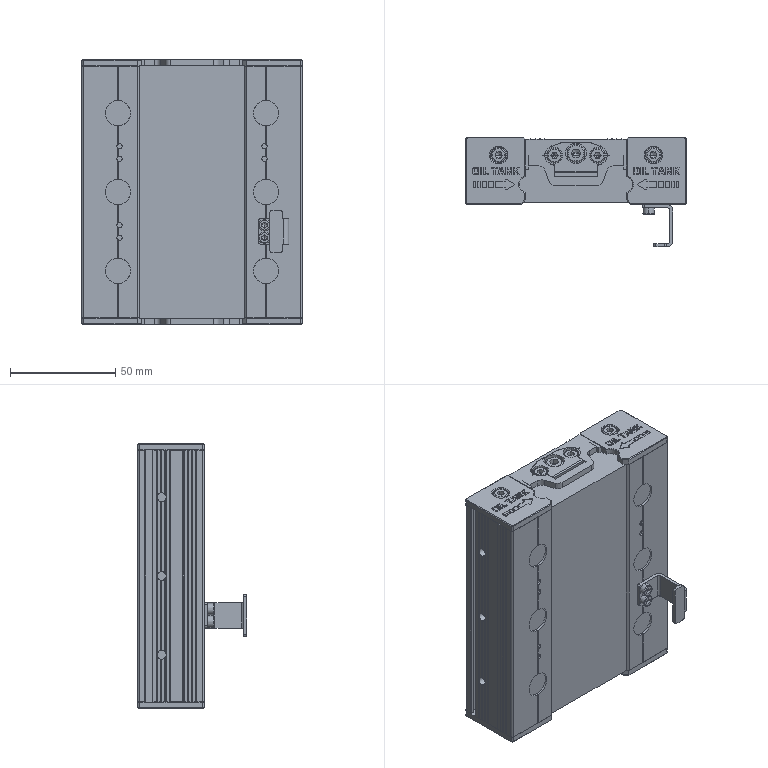Part | SolidWorks | features BaseBody 4 | 4 solids | 1989 faces | box 105 x 52 x 126 mm | volume 392725 mm3 | plane 1239 | cylinder 543 | cone 137 | torus 38 | spline 32 | commonest cylinder face diameters 0.2 x131 0.4 x95 2 x38 7 x30 8 x25 4.2 x22